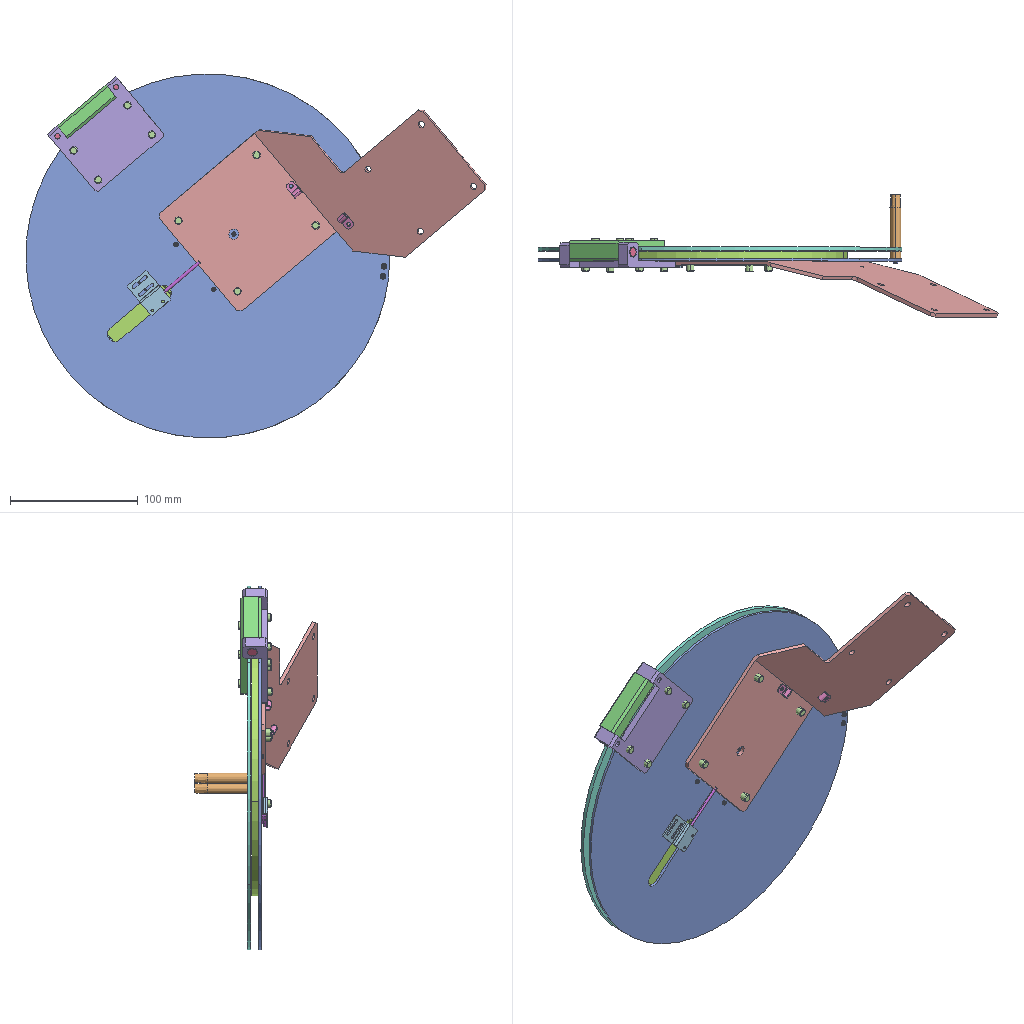Assembly | SolidWorks | 17 different items | 39 placed | box 360 x 96 x 285 mm
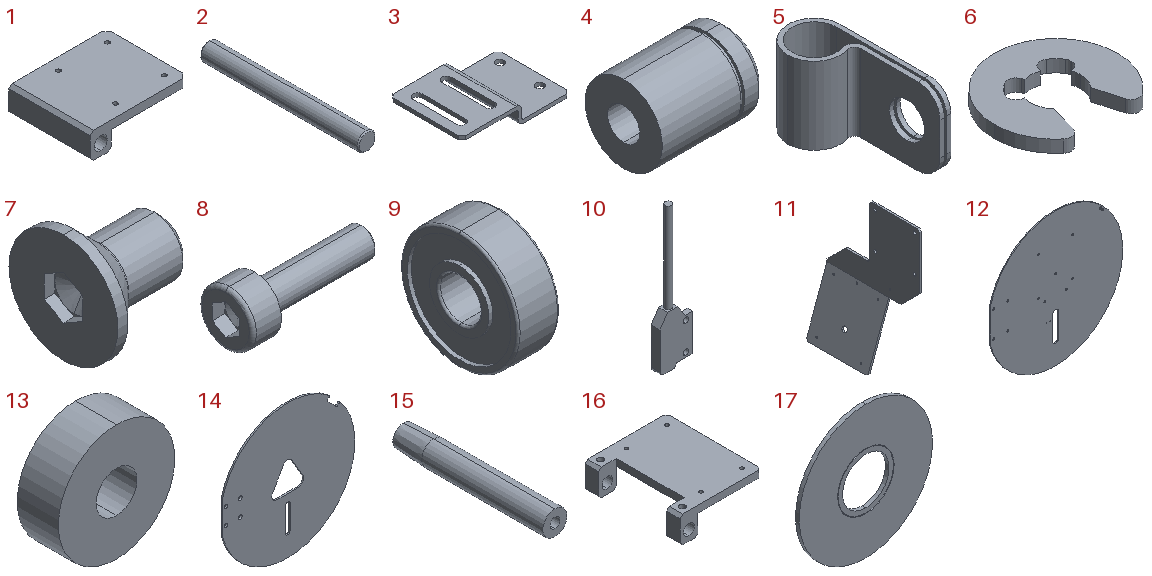Parts list (item | quantity | size | volume | features):
1 | x1 | 60 x 50 x 16 mm | 19181 mm3 | features Chamfer 3, ICE 2, 3DProfileFeature 1, Extrusion 1, HoleWzd 1, LPattern 1
2 | x1 | 8 x 70 x 8 mm | 3487 mm3 | features Chamfer 1, Extrusion 1, ICE 1
3 | x1 | 30 x 20 x 5 mm | 583.412 mm3 | features Fillet 2, Chamfer 1, Extrusion 1, HoleWzd 1, ICE 1
4 | x3 | 8 x 6 x 6 mm | 189.74 mm3 | features 3DProfileFeature 1, Chamfer 1, Extrusion 1, HoleWzd 1, RevCut 1
5 | x2 | 4.8 x 12.4 x 7 mm | 75.143 mm3 | features Extrusion 1, Fillet 1, ICE 1
6 | x3 | 3 x 2.7 x 0.3 mm | 1.322 mm3 | features Extrusion 1
7 | x12 | 10 x 11.34 x 11.34 mm | 423.495 mm3 | features RevCut 3, Chamfer 1, Cut 1, Fillet 1, LPattern 1, Revolution 1
8 | x5 | 7.6 x 3 x 3 mm | 21.652 mm3 | features Fillet 2, RevCut 2, Boss 1, Chamfer 1, Cut 1, Extrusion 1, LPattern 1
9 | x2 | 6 x 17 x 17 mm | 1055 mm3 | features RefAxis 6, 3DProfileFeature 2, Revolution 1
10 | x1 | 13 x 4 x 56 mm | 912.44 mm3 | features ICE 4, Chamfer 2, Fillet 2, Extrusion 1
11 | x1 | 37.021 x 150 x 213.969 mm | 62969 mm3 | features Chamfer 4, ICE 4, HoleWzd 3, 3DProfileFeature 1, Cut 1, Extrusion 1, Fillet 1, LPattern 1
12 | x1 | 280.5 x 2 x 285 mm | 125189 mm3 | features ICE 3, Chamfer 2, Cut 2, 3DProfileFeature 1, CirPattern 1, Extrusion 1, HoleWzd 1
13 | x1 | 17 x 6 x 17 mm | 1192 mm3 | features Extrusion 1
14 | x1 | 280.5 x 3 x 285 mm | 179414 mm3 | features ICE 5, Chamfer 1, CirPattern 1, Cut 1, Extrusion 1, Fillet 1
15 | x2 | 8 x 50 x 8 mm | 2364 mm3 | features Chamfer 1, Extrusion 1, HoleWzd 1
16 | x1 | 60 x 70 x 19.5 mm | 20039 mm3 | features ICE 6, 3DProfileFeature 3, Chamfer 3, HoleWzd 3, Extrusion 1, LPattern 1
17 | x1 | 200 x 5.5 x 200 mm | 151356 mm3 | features Chamfer 1, Extrusion 1, ICE 1
Mates (type | each side: item.copy, entity, surface, feature):
Coincident | 12.1 face plane Boss-Extrude1 | 17.1 face plane Boss-Extrude2
Concentric | 12.1 face cylinder Boss-Extrude1 | 17.1 face cylinder Boss-Extrude2
Coincident | 12.1 face plane Boss-Extrude1 | 9.1 face plane Revolve1
Concentric | 12.1 face cylinder CirPattern1 | 9.1 face cylinder Revolve1
Concentric | 12.1 face cylinder CirPattern1 | 9.2 face cylinder Revolve1
Coincident | 12.1 face plane Boss-Extrude1 | 9.2 face plane Revolve1
Coincident | 12.1 face plane Boss-Extrude1 | 13.1 face plane Boss-Extrude1
Concentric | 12.1 face cylinder Cut-Extrude1 | 13.1 face cylinder Boss-Extrude1
PlanarAngleDim | 14.1 plane | 11.1 face plane Boss-Extrude1
Coincident | 12.1 face plane Boss-Extrude1 | 15.1 face plane Boss-Extrude1
Coincident | 12.1 face plane Boss-Extrude1 | 15.2 face plane Boss-Extrude1
Coincident | 12.1 face plane Boss-Extrude1 | 16.1 face plane Boss-Extrude1
Concentric | 12.1 face cylinder Cut-Extrude2 | 15.2 face cylinder Boss-Extrude1
Concentric | 12.1 face cylinder Cut-Extrude2 | 15.1 face cylinder Boss-Extrude1
Coincident | 16.1 face plane Cut-Extrude2 | 1.1 face plane Boss-Extrude1
Concentric | 16.1 face cylinder Cut-Extrude3 | 2.1 face cylinder Boss-Extrude1
Coincident | 16.1 face plane Boss-Extrude1 | 2.1 face plane Boss-Extrude1
Concentric | 1.1 face cylinder Cut-Extrude2 | 2.1 face cylinder Boss-Extrude1
Coincident | 14.1 face plane Boss-Extrude1 | 1.1 face plane Boss-Extrude1
Coincident | 3.1 face plane Boss-Extrude1 | 10.1 face plane Boss-Extrude1 | 3 times
DistanceDim | 3.1 face plane Boss-Extrude1 | 11.1 face plane Boss-Extrude1
Coincident | 12.1 face plane Boss-Extrude1 | 7.1 face plane Base
Concentric | 12.1 face cylinder Cut-Extrude4 | 7.1 face cylinder Base
Coincident | 12.1 face plane Boss-Extrude1 | 7.2 face plane Base
Concentric | 12.1 face cylinder Cut-Extrude4 | 7.2 face cylinder Base
Coincident | 12.1 face plane Boss-Extrude1 | 7.3 face plane Base
Concentric | 12.1 face cylinder Cut-Extrude4 | 7.3 face cylinder Base
DistanceDim | 12.1 face plane Boss-Extrude1 | 7.4 face plane Base
Concentric | 12.1 edge | 7.4 face cylinder Base
Coincident | 12.1 face plane Boss-Extrude1 | 4.1 face plane Boss-Extrude1
Concentric | 12.1 face cylinder CirPattern1 | 4.1 face cylinder Boss-Extrude1
Coincident | 12.1 face plane Boss-Extrude1 | 4.2 face plane Boss-Extrude1
Concentric | 12.1 face cylinder CirPattern1 | 4.2 face cylinder Boss-Extrude1
Coincident | 12.1 face plane Boss-Extrude1 | 4.3 face plane Boss-Extrude1
Concentric | 12.1 face cylinder Cut-Extrude1 | 4.3 face cylinder Boss-Extrude1
Concentric | 4.1 face cylinder Cut-Revolve1 | 6.1 face cylinder Body
Coincident | 4.1 face plane Cut-Revolve1 | 6.1 face plane Body
Coincident | 4.3 face plane Cut-Revolve1 | 6.2 face plane Body
Concentric | 4.3 face cylinder Boss-Extrude1 | 6.2 face cylinder Body
Coincident | 4.2 face plane Cut-Revolve1 | 6.3 face plane Body
Concentric | 4.2 face cylinder Boss-Extrude1 | 6.3 face cylinder Body
Concentric | 11.1 face cylinder M3 Tapped Hole1 | 7.4 face cylinder Base
Concentric | 11.1 face cylinder M3 Tapped Hole1 | 7.3 face cylinder Base
Coincident | 11.1 face plane Boss-Extrude1 | 12.1 face plane Boss-Extrude1
Concentric | 12.1 face cylinder Boss-Extrude1 | 14.1 face cylinder Boss-Extrude1
Concentric | 12.1 face cylinder Cut-Extrude2 | 8.1 face cylinder BaseBody
Coincident | 12.1 face plane Boss-Extrude1 | 8.1 face plane BaseHead
Concentric | 12.1 face cylinder Cut-Extrude2 | 8.2 face cylinder BaseBody
Coincident | 12.1 face plane Boss-Extrude1 | 8.2 face plane BaseHead
Concentric | 12.1 face cone Chamfer2 | 7.5 face cylinder Cut-Revolve2
Coincident | 12.1 face plane Boss-Extrude1 | 7.5 face plane Base
Concentric | 12.1 face cone Chamfer2 | 7.6 face cylinder Cut-Revolve2
Coincident | 12.1 face plane Boss-Extrude1 | 7.6 face plane Base
Concentric | 12.1 face cone Chamfer2 | 7.7 face cylinder Cut-Revolve2
Coincident | 12.1 face plane Boss-Extrude1 | 7.7 face plane Base
Concentric | 12.1 face cone Chamfer2 | 7.8 face cylinder Cut-Revolve2
DistanceDim | 12.1 face plane Boss-Extrude1 | 7.8 face plane Base
Concentric | 1.1 face cylinder M3 Tapped Hole1 | 7.9 face cylinder Cut-Revolve2
Concentric | 1.1 face cylinder M3 Tapped Hole1 | 7.10 face cylinder Cut-Revolve2
Concentric | 1.1 face cylinder M3 Tapped Hole1 | 7.11 face cylinder Cut-Revolve2
Concentric | 1.1 face cylinder M3 Tapped Hole1 | 7.12 face cylinder Cut-Revolve2
Concentric | 16.1 face cylinder M3 Tapped Hole1 | 7.5 face cylinder Base
Concentric | 16.1 face cylinder M3 Tapped Hole1 | 7.8 face cylinder Base
Coincident | 14.1 face plane Boss-Extrude1 | 7.12 face plane Base
Coincident | 14.1 face plane Boss-Extrude1 | 7.11 face plane Base
Coincident | 14.1 face plane Boss-Extrude1 | 7.9 face plane Base
Coincident | 14.1 face plane Boss-Extrude1 | 7.10 face plane Base
Coincident | 12.1 face plane Boss-Extrude1 | 3.1 face plane Boss-Extrude1
Coincident | 12.1 face plane Cut-Extrude3 | 3.1 face plane Boss-Extrude1
Concentric | 12.1 face cylinder CirPattern1 | 8.3 face cylinder BaseBody
Coincident | 12.1 face plane Boss-Extrude1 | 8.3 face plane BaseHead
Concentric | 12.1 face cylinder CirPattern1 | 8.4 face cylinder BaseBody
Coincident | 12.1 face plane Boss-Extrude1 | 8.4 face plane BaseHead
Concentric | 12.1 face cylinder Cut-Extrude1 | 8.5 face cylinder BaseBody
Coincident | 12.1 face plane Boss-Extrude1 | 8.5 face plane BaseHead
Coincident | 11.1 face plane Boss-Extrude1 | 5.1 face plane Boss-Extrude1
Concentric | 11.1 face cylinder M3 Tapped Hole2 | 5.1 face cylinder Cut-Extrude1
Coincident | 11.1 face plane Boss-Extrude1 | 5.2 face plane Boss-Extrude1
Concentric | 11.1 face cylinder M3 Tapped Hole3 | 5.2 face cylinder Cut-Extrude1
Parallel | 11.1 face plane Boss-Extrude2 | 5.2 face plane Boss-Extrude1